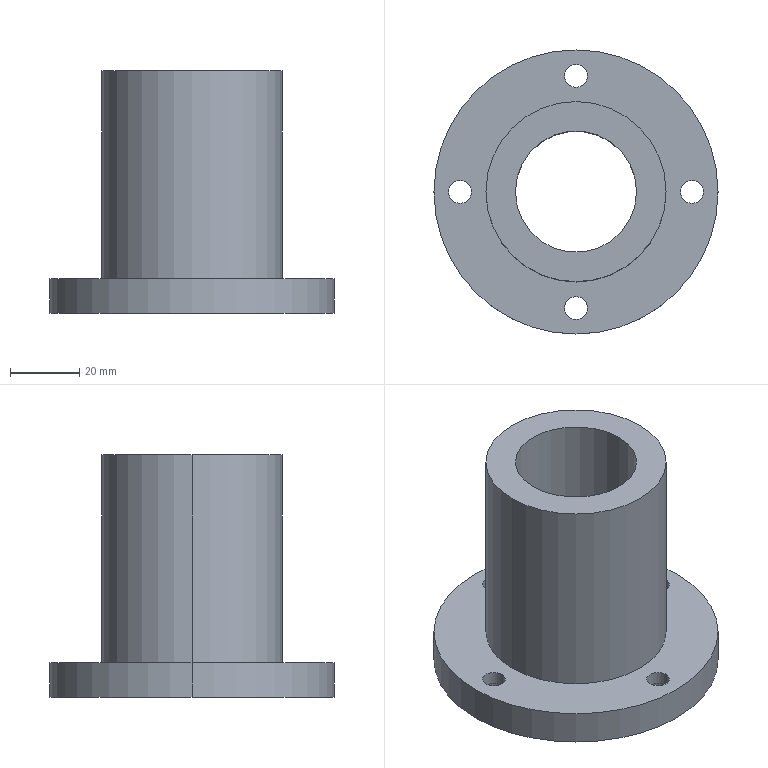Part | STEP file | LHFRD35 | 1 solid | 29 faces | box 82 x 82 x 70 mm | volume 110033 mm3 | cylinder 22 | plane 7 | commonest cylinder face diameters 6.6 x8 11 x8 35 x2 52 x2 82 x2